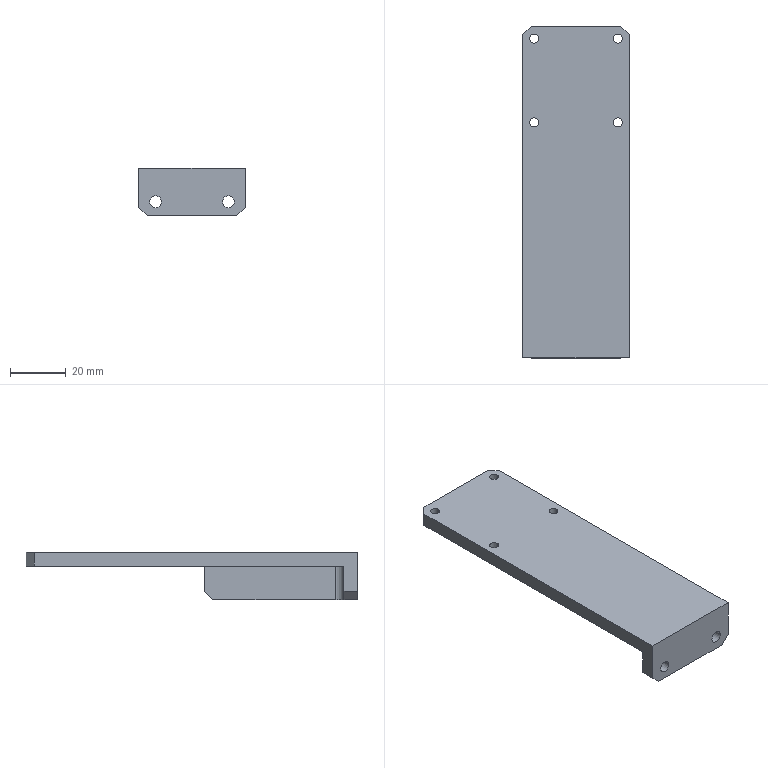NC program | NX | posted with a generic post | part box 38.1 x 118.8 x 17 mm
Lines 1974 to 2704 of 2704:
(ZLEVEL_PROFILE_1 , TOOL : D6R0.5)
N3916 T16 M6
N3918 G54
N3920 G17 G0 G90 X-2.413 Y7.413 S9500 M3
N3922 G43 Z30. H16
N3924 Z2.929
N3926 G94 G1 Z-0.071 F3500.
N3928 G3 X-4.625 Y4.472 R3.
N3930 G1 X-4.622 Y4.301
N3932 Y-4.301
N3934 X-4.625 Y-4.472
N3936 X-4.587 Y-4.473 Z-0.106
N3938 X-4.554 Z-0.141
N3940 X-4.551 Y-4.301
N3942 Y4.301
N3944 X-4.554 Y4.473
N3946 X-4.516 Z-0.177
N3948 X-4.483 Z-0.212
N3950 X-4.481 Y4.
N3952 Y-4.
N3954 X-4.483 Y-4.473
N3956 X-4.445 Z-0.247
N3958 X-4.413 Y-4.474 Z-0.283
N3960 X-4.41 Y-4.
N3962 Y4.
N3964 X-4.413 Y4.473
N3966 X-4.375 Y4.474 Z-0.318
N3968 X-4.342 Z-0.354
N3970 X-4.339 Y4.
N3972 Y-4.
N3974 X-4.342 Y-4.474
N3976 X-4.304 Z-0.389
N3978 X-4.271 Z-0.424
N3980 X-4.269 Y-4.
N3982 Y4.
N3984 X-4.271 Y4.474
N3986 X-4.233 Z-0.46
N3988 X-4.2 Y4.475 Z-0.495
N3990 X-4.198 Y4.
N3992 Y-4.
N3994 X-4.2 Y-4.475
N3996 X-4.163 Z-0.53
N3998 X-4.13 Z-0.566
N4000 X-4.127 Y-4.
N4002 Y4.
N4004 X-4.13 Y4.475
N4006 X-4.092 Z-0.601
N4008 X-4.059 Z-0.636
N4010 X-4.056 Y4.
N4012 Y-4.
N4014 X-4.059 Y-4.475
N4016 X-4.021 Y-4.476 Z-0.672
N4018 X-3.988 Z-0.707
N4020 X-3.986 Y-4.
N4022 Y4.
N4024 X-3.988 Y4.476
N4026 X-3.95 Z-0.742
N4028 X-3.918 Z-0.778
N4030 X-3.915 Y4.
N4032 Y-4.
N4034 X-3.918 Y-4.476
N4036 X-3.88 Z-0.813
N4038 X-3.847 Y-4.477 Z-0.849
N4040 X-3.844 Y-4.
N4042 Y4.
N4044 X-3.847 Y4.477
N4046 X-3.809 Z-0.884
N4048 X-3.776 Z-0.919
N4050 X-3.774 Y4.
N4052 Y-4.
N4054 X-3.776 Y-4.477
N4056 X-3.738 Z-0.955
N4058 X-3.705 Z-0.99
N4060 X-3.703 Y-4.
N4062 Y4.
N4064 X-3.705 Y4.477
N4066 X-3.668 Y4.478 Z-1.025
N4068 X-3.635 Z-1.061
N4070 X-3.632 Y4.
N4072 Y-4.
N4074 X-3.635 Y-4.478
N4076 X-3.597 Z-1.096
N4078 X-3.564 Z-1.131
N4080 X-3.562 Y-4.
N4082 Y4.
N4084 X-3.564 Y4.478
N4086 X-3.526 Z-1.167
N4088 X-3.493 Z-1.202
N4090 X-3.491 Y4.
N4092 Y-4.
N4094 X-3.493 Y-4.478
N4096 X-3.455 Z-1.237
N4098 X-3.423 Z-1.273
N4100 X-3.42 Y-4.
N4102 Y4.
N4104 X-3.423 Y4.478
N4106 X-3.385 Z-1.308
N4108 X-3.352 Z-1.344
N4110 X-3.349 Y4.
N4112 Y-4.
N4114 X-3.352 Y-4.478
N4116 X-3.314 Z-1.379
N4118 X-3.281 Z-1.414
N4120 X-3.279 Y-4.
N4122 Y4.
N4124 X-3.281 Y4.478
N4126 X-3.243 Z-1.45
N4128 X-3.21 Z-1.485
N4130 X-3.208 Y4.
N4132 Y-4.
N4134 X-3.21 Y-4.478
N4136 X-3.173 Z-1.52
N4138 X-3.14 Z-1.556
N4140 X-3.137 Y-4.
N4142 Y4.
N4144 X-3.14 Y4.478
N4146 X-3.102 Z-1.591
N4148 X-3.069 Z-1.626
N4150 X-3.067 Y4.
N4152 Y-4.
N4154 X-3.069 Y-4.478
N4156 X-3.031 Z-1.662
N4158 X-2.998 Z-1.697
N4160 X-2.996 Y-4.
N4162 Y4.
N4164 X-2.998 Y4.478
N4166 X-2.96 Z-1.732
N4168 X-2.928 Z-1.768
N4170 X-2.925 Y4.
N4172 Y-4.
N4174 X-2.928 Y-4.478
N4176 X-2.89 Z-1.803
N4178 X-2.857 Z-1.838
N4180 X-2.854 Y-4.
N4182 Y4.
N4184 X-2.857 Y4.478
N4186 X-2.819 Z-1.874
N4188 X-2.786 Z-1.909
N4190 X-2.784 Y4.
N4192 Y-4.
N4194 X-2.786 Y-4.478
N4196 X-2.748 Z-1.945
N4198 X-2.716 Z-1.98
N4200 X-2.713 Y-4.
N4202 Y4.
N4204 X-2.716 Y4.478
N4206 X-2.678 Z-2.015
N4208 X-2.645 Z-2.051
N4210 X-2.642 Y4.
N4212 Y-4.
N4214 X-2.645 Y-4.478
N4216 X-2.607 Z-2.086
N4218 X-2.574 Z-2.121
N4220 X-2.572 Y-4.
N4222 Y4.
N4224 X-2.574 Y4.478
N4226 X-2.536 Z-2.157
N4228 X-2.503 Z-2.192
N4230 X-2.501 Y4.
N4232 Y-4.
N4234 X-2.503 Y-4.478
N4236 X-2.466 Y-4.477 Z-2.227
N4238 X-2.433 Z-2.263
N4240 X-2.43 Y-4.
N4242 Y4.
N4244 X-2.433 Y4.477
N4246 X-2.395 Z-2.298
N4248 X-2.362 Z-2.333
N4250 X-2.359 Y4.
N4252 Y-4.
N4254 X-2.362 Y-4.477
N4256 X-2.324 Z-2.369
N4258 X-2.291 Z-2.404
N4260 X-2.289 Y-4.
N4262 Y4.
N4264 X-2.291 Y4.477
N4266 X-2.253 Z-2.44
N4268 X-2.221 Y4.476 Z-2.475
N4270 X-2.218 Y4.
N4272 Y-4.
N4274 X-2.221 Y-4.476
N4276 X-2.183 Z-2.51
N4278 X-2.15 Z-2.546
N4280 X-2.147 Y-4.
N4282 Y4.
N4284 X-2.15 Y4.476
N4286 X-2.112 Z-2.581
N4288 X-2.079 Z-2.616
N4290 X-2.077 Y4.
N4292 Y-4.
N4294 X-2.079 Y-4.476
N4296 X-2.041 Y-4.475 Z-2.652
N4298 X-2.008 Z-2.687
N4300 X-2.006 Y-4.
N4302 Y4.
N4304 X-2.008 Y4.475
N4306 X-1.971 Z-2.722
N4308 X-1.938 Z-2.758
N4310 X-1.935 Y4.
N4312 Y-4.
N4314 X-1.938 Y-4.475
N4316 X-1.9 Z-2.793
N4318 X-1.867 Y-4.474 Z-2.828
N4320 X-1.864 Y-4.
N4322 Y4.
N4324 X-1.867 Y4.474
N4326 X-1.829 Z-2.864
N4328 X-1.796 Z-2.899
N4330 X-1.794 Y4.
N4332 Y-4.
N4334 X-1.796 Y-4.474
N4336 X-1.758 Z-2.934
N4338 X-1.726 Z-2.97
N4340 X-1.723 Y-4.
N4342 Y4.
N4344 X-1.726 Y4.474
N4346 X-1.688 Y4.473 Z-3.005
N4348 X-1.655 Z-3.041
N4350 X-1.652 Y4.
N4352 Y-4.
N4354 X-1.655 Y-4.473
N4356 X-1.617 Z-3.076
N4358 X-1.584 Z-3.111
N4360 X-1.582 Y-4.
N4362 Y4.
N4364 X-1.584 Y4.473
N4366 X-1.546 Z-3.147
N4368 X-1.514 Y4.472 Z-3.182
N4370 X-1.511 Y4.301
N4372 Y-4.301
N4374 X-1.514 Y-4.472
N4376 X-1.476 Z-3.217
N4378 X-1.443 Z-3.253
N4380 X-1.44 Y-4.301
N4382 Y4.301
N4384 X-1.443 Y4.472
N4386 X-1.409 Z-3.284
N4388 X-1.381 Z-3.315
N4390 X-1.378 Y4.301
N4392 Y-4.301
N4394 X-1.381 Y-4.472
N4396 X-1.347 Y-4.471 Z-3.345
N4398 X-1.319 Z-3.376
N4400 X-1.317 Y-4.301
N4402 Y4.301
N4404 X-1.319 Y4.471
N4406 X-1.256 Y4.391 Z-3.438
N4408 X-1.255 Y4.301
N4410 Y-4.301
N4412 X-1.256 Y-4.391
N4414 G3 X0.989 Y-7.351 R3.
N4416 G1 Z-0.438
N4418 G0 Z30.
N4420 X-51.024 Y-21.059
N4422 Z2.929
N4424 G1 Z-0.071
N4426 G3 X-53.968 Y-18.826 R3.
N4428 G1 X-54.106 Y-18.828
N4430 X-59.815 Y-18.827
N4432 X-59.869 Y-18.898 Z-0.141
N4434 X-54.106 Y-18.899
N4436 X-53.93 Y-18.896
N4438 X-53.928 Y-18.934 Z-0.177
N4440 X-53.927 Y-18.967 Z-0.212
N4442 X-54.4 Y-18.969
N4444 X-59.4
N4446 X-59.873 Y-18.968
N4448 Y-19.005 Z-0.247
N4450 X-59.874 Y-19.039 Z-0.283
N4452 X-59.4 Y-19.04
N4454 X-54.4
N4456 X-53.927 Y-19.037
N4458 X-53.926 Y-19.075 Z-0.318
N4460 Y-19.108 Z-0.354
N4462 X-54.4 Y-19.111
N4464 X-59.4
N4466 X-59.874 Y-19.11
N4468 Y-19.146 Z-0.389
N4470 Y-19.18 Z-0.424
N4472 X-59.4 Y-19.181
N4474 X-54.4
N4476 X-53.926 Y-19.179
N4478 Y-19.217 Z-0.46
N4480 X-53.925 Y-19.25 Z-0.495
N4482 X-54.4 Y-19.252
N4484 X-59.4
N4486 X-59.875 Y-19.251
N4488 Y-19.287 Z-0.53
N4490 Y-19.322 Z-0.566
N4492 X-59.4 Y-19.323
N4494 X-54.4
N4496 X-53.925 Y-19.32
N4498 Y-19.358 Z-0.601
N4500 Y-19.391 Z-0.636
N4502 X-54.4 Y-19.394
N4504 X-59.4
N4506 X-59.875 Y-19.393
N4508 X-59.876 Y-19.429 Z-0.672
N4510 Y-19.463 Z-0.707
N4512 X-59.4 Y-19.464
N4514 X-54.4
N4516 X-53.924 Y-19.462
N4518 Y-19.5 Z-0.742
N4520 Y-19.532 Z-0.778
N4522 X-54.4 Y-19.535
N4524 X-59.4
N4526 X-59.876 Y-19.534
N4528 Y-19.57 Z-0.813
N4530 X-59.877 Y-19.605 Z-0.849
N4532 X-59.4 Y-19.606
N4534 X-54.4
N4536 X-53.923 Y-19.603
N4538 Y-19.641 Z-0.884
N4540 Y-19.674 Z-0.919
N4542 X-54.4 Y-19.676
N4544 X-59.4
N4546 X-59.877 Y-19.675
N4548 Y-19.712 Z-0.955
N4550 Y-19.746 Z-0.99
N4552 X-59.4 Y-19.747
N4554 X-54.4
N4556 X-53.923 Y-19.745
N4558 X-53.922 Y-19.782 Z-1.025
N4560 Y-19.815 Z-1.061
N4562 X-54.4 Y-19.818
N4564 X-59.4
N4566 X-59.878 Y-19.817
N4568 Y-19.853 Z-1.096
N4570 Y-19.888 Z-1.131
N4572 X-59.4
N4574 X-54.4
N4576 X-53.922 Y-19.886
N4578 Y-19.924 Z-1.167
N4580 Y-19.957 Z-1.202
N4582 X-54.4 Y-19.959
N4584 X-59.4
N4586 X-59.878 Y-19.958
N4588 Y-19.995 Z-1.237
N4590 Y-20.029 Z-1.273
N4592 X-59.4 Y-20.03
N4594 X-54.4
N4596 X-53.922 Y-20.027
N4598 Y-20.065 Z-1.308
N4600 Y-20.098 Z-1.344
N4602 X-54.4 Y-20.101
N4604 X-59.4
N4606 X-59.878 Y-20.1
N4608 Y-20.136 Z-1.379
N4610 Y-20.17 Z-1.414
N4612 X-59.4 Y-20.171
N4614 X-54.4
N4616 X-53.922 Y-20.169
N4618 Y-20.207 Z-1.45
N4620 Y-20.24 Z-1.485
N4622 X-54.4 Y-20.242
N4624 X-59.4
N4626 X-59.878 Y-20.241
N4628 Y-20.277 Z-1.52
N4630 Y-20.312 Z-1.556
N4632 X-59.4 Y-20.313
N4634 X-54.4
N4636 X-53.922 Y-20.31
N4638 Y-20.348 Z-1.591
N4640 Y-20.381 Z-1.626
N4642 X-54.4 Y-20.383
N4644 X-59.4
N4646 X-59.878
N4648 Y-20.419 Z-1.662
N4650 Y-20.453 Z-1.697
N4652 X-59.4 Y-20.454
N4654 X-54.4
N4656 X-53.922 Y-20.452
N4658 Y-20.49 Z-1.732
N4660 Y-20.522 Z-1.768
N4662 X-54.4 Y-20.525
N4664 X-59.4
N4666 X-59.878 Y-20.524
N4668 Y-20.56 Z-1.803
N4670 Y-20.595 Z-1.838
N4672 X-59.4 Y-20.596
N4674 X-54.4
N4676 X-53.922 Y-20.593
N4678 Y-20.631 Z-1.874
N4680 Y-20.664 Z-1.909
N4682 X-54.4 Y-20.666
N4684 X-59.4
N4686 X-59.878 Y-20.665
N4688 Y-20.702 Z-1.945
N4690 Y-20.736 Z-1.98
N4692 X-59.4 Y-20.737
N4694 X-54.4
N4696 X-53.922 Y-20.735
N4698 Y-20.772 Z-2.015
N4700 Y-20.805 Z-2.051
N4702 X-54.4 Y-20.808
N4704 X-59.4
N4706 X-59.878 Y-20.807
N4708 Y-20.843 Z-2.086
N4710 Y-20.878 Z-2.121
N4712 X-59.4
N4714 X-54.4
N4716 X-53.922 Y-20.876
N4718 Y-20.914 Z-2.157
N4720 Y-20.947 Z-2.192
N4722 X-54.4 Y-20.949
N4724 X-59.4
N4726 X-59.878 Y-20.948
N4728 Y-20.984 Z-2.227
N4730 Y-21.019 Z-2.263
N4732 X-59.4 Y-21.02
N4734 X-54.4
N4736 X-53.922 Y-21.017
N4738 X-53.923 Y-21.055 Z-2.298
N4740 Y-21.088 Z-2.333
N4742 X-54.4 Y-21.091
N4744 X-59.4
N4746 X-59.877 Y-21.09
N4748 Y-21.126 Z-2.369
N4750 Y-21.16 Z-2.404
N4752 X-59.4 Y-21.161
N4754 X-54.4
N4756 X-53.923 Y-21.159
N4758 Y-21.197 Z-2.44
N4760 X-53.924 Y-21.23 Z-2.475
N4762 X-54.4 Y-21.232
N4764 X-59.4
N4766 X-59.876 Y-21.231
N4768 Y-21.267 Z-2.51
N4770 Y-21.302 Z-2.546
N4772 X-59.4 Y-21.303
N4774 X-54.4
N4776 X-53.924 Y-21.3
N4778 Y-21.338 Z-2.581
N4780 Y-21.371 Z-2.616
N4782 X-54.4 Y-21.373
N4784 X-59.4
N4786 X-59.876 Y-21.372
N4788 X-59.875 Y-21.409 Z-2.652
N4790 Y-21.443 Z-2.687
N4792 X-59.4 Y-21.444
N4794 X-54.4
N4796 X-53.925 Y-21.442
N4798 Y-21.479 Z-2.722
N4800 Y-21.512 Z-2.758
N4802 X-54.4 Y-21.515
N4804 X-59.4
N4806 X-59.875 Y-21.514
N4808 Y-21.55 Z-2.793
N4810 Y-21.585 Z-2.828
N4812 X-59.4 Y-21.586
N4814 X-54.4
N4816 X-53.926 Y-21.583
N4818 Y-21.621 Z-2.864
N4820 Y-21.654 Z-2.899
N4822 X-54.4 Y-21.656
N4824 X-59.4
N4826 X-59.874 Y-21.655
N4828 Y-21.692 Z-2.934
N4830 Y-21.726 Z-2.97
N4832 X-59.4 Y-21.727
N4834 X-54.4
N4836 X-53.926 Y-21.724
N4838 X-53.927 Y-21.762 Z-3.005
N4840 Y-21.795 Z-3.041
N4842 X-54.4 Y-21.798
N4844 X-59.4
N4846 X-59.873 Y-21.797
N4848 Y-21.833 Z-3.076
N4850 Y-21.867 Z-3.111
N4852 X-59.4 Y-21.868
N4854 X-54.4
N4856 X-53.927 Y-21.866
N4858 Y-21.904 Z-3.147
N4860 X-53.928 Y-21.937 Z-3.182
N4862 X-54.106 Y-21.939
N4864 X-59.873 Y-21.938
N4866 X-59.872 Y-21.974 Z-3.217
N4868 Y-22.009 Z-3.253
N4870 X-54.106 Y-22.01
N4872 X-53.928 Y-22.007
N4874 X-53.974 Y-22.07 Z-3.315
N4876 X-54.106 Y-22.072
N4878 X-59.806 Y-22.071
N4880 X-59.735 Y-22.133 Z-3.376
N4882 X-54.023 Y-22.132
N4884 X-54.072 Y-22.195 Z-3.438
N4886 X-59.664
N4888 G3 X-62.588 Y-24.526 R3.
N4890 G1 Z-0.438
N4892 G0 Z30.
N4894 X-62.722 Y21.085
N4896 Z2.929
N4898 G1 Z-0.071
N4900 G3 X-59.815 Y18.827 R3.
N4902 G1 X-54.106 Y18.828
N4904 X-53.968 Y18.826
N4906 X-53.93 Y18.896 Z-0.141
N4908 X-54.106 Y18.899
N4910 X-59.869 Y18.898
N4912 X-59.871 Y18.934 Z-0.177
N4914 X-59.873 Y18.968 Z-0.212
N4916 X-59.4 Y18.969
N4918 X-54.4
N4920 X-53.927 Y18.967
N4922 Y19.005 Z-0.247
N4924 Y19.037 Z-0.283
N4926 X-54.4 Y19.04
N4928 X-59.4
N4930 X-59.874 Y19.039
N4932 Y19.075 Z-0.318
N4934 Y19.11 Z-0.354
N4936 X-59.4 Y19.111
N4938 X-54.4
N4940 X-53.926 Y19.108
N4942 Y19.146 Z-0.389
N4944 Y19.179 Z-0.424
N4946 X-54.4 Y19.181
N4948 X-59.4
N4950 X-59.874 Y19.18
N4952 X-59.875 Y19.217 Z-0.46
N4954 Y19.251 Z-0.495
N4956 X-59.4 Y19.252
N4958 X-54.4
N4960 X-53.925 Y19.25
N4962 Y19.287 Z-0.53
N4964 Y19.32 Z-0.566
N4966 X-54.4 Y19.323
N4968 X-59.4
N4970 X-59.875 Y19.322
N4972 Y19.358 Z-0.601
N4974 Y19.393 Z-0.636
N4976 X-59.4 Y19.394
N4978 X-54.4
N4980 X-53.925 Y19.391
N4982 X-53.924 Y19.429 Z-0.672
N4984 Y19.462 Z-0.707
N4986 X-54.4 Y19.464
N4988 X-59.4
N4990 X-59.876 Y19.463
N4992 Y19.5 Z-0.742
N4994 Y19.534 Z-0.778
N4996 X-59.4 Y19.535
N4998 X-54.4
N5000 X-53.924 Y19.532
N5002 Y19.57 Z-0.813
N5004 X-53.923 Y19.603 Z-0.849
N5006 X-54.4 Y19.606
N5008 X-59.4
N5010 X-59.877 Y19.605
N5012 Y19.641 Z-0.884
N5014 Y19.675 Z-0.919
N5016 X-59.4 Y19.676
N5018 X-54.4
N5020 X-53.923 Y19.674
N5022 Y19.712 Z-0.955
N5024 Y19.745 Z-0.99
N5026 X-54.4 Y19.747
N5028 X-59.4
N5030 X-59.877 Y19.746
N5032 Y19.782 Z-1.025
N5034 X-59.878 Y19.817 Z-1.061
N5036 X-59.4 Y19.818
N5038 X-54.4
N5040 X-53.922 Y19.815
N5042 Y19.853 Z-1.096
N5044 Y19.886 Z-1.131
N5046 X-54.4 Y19.888
N5048 X-59.4
N5050 X-59.878
N5052 Y19.924 Z-1.167
N5054 Y19.958 Z-1.202
N5056 X-59.4 Y19.959
N5058 X-54.4
N5060 X-53.922 Y19.957
N5062 Y19.995 Z-1.237
N5064 Y20.027 Z-1.273
N5066 X-54.4 Y20.03
N5068 X-59.4
N5070 X-59.878 Y20.029
N5072 Y20.065 Z-1.308
N5074 Y20.1 Z-1.344
N5076 X-59.4 Y20.101
N5078 X-54.4
N5080 X-53.922 Y20.098
N5082 Y20.136 Z-1.379
N5084 Y20.169 Z-1.414
N5086 X-54.4 Y20.171
N5088 X-59.4
N5090 X-59.878 Y20.17
N5092 Y20.207 Z-1.45
N5094 Y20.241 Z-1.485
N5096 X-59.4 Y20.242
N5098 X-54.4
N5100 X-53.922 Y20.24
N5102 Y20.277 Z-1.52
N5104 Y20.31 Z-1.556
N5106 X-54.4 Y20.313
N5108 X-59.4
N5110 X-59.878 Y20.312
N5112 Y20.348 Z-1.591
N5114 Y20.383 Z-1.626
N5116 X-59.4
N5118 X-54.4
N5120 X-53.922 Y20.381
N5122 Y20.419 Z-1.662
N5124 Y20.452 Z-1.697
N5126 X-54.4 Y20.454
N5128 X-59.4
N5130 X-59.878 Y20.453
N5132 Y20.49 Z-1.732
N5134 Y20.524 Z-1.768
N5136 X-59.4 Y20.525
N5138 X-54.4
N5140 X-53.922 Y20.522
N5142 Y20.56 Z-1.803
N5144 Y20.593 Z-1.838
N5146 X-54.4 Y20.596
N5148 X-59.4
N5150 X-59.878 Y20.595
N5152 Y20.631 Z-1.874
N5154 Y20.665 Z-1.909
N5156 X-59.4 Y20.666
N5158 X-54.4
N5160 X-53.922 Y20.664
N5162 Y20.702 Z-1.945
N5164 Y20.735 Z-1.98
N5166 X-54.4 Y20.737
N5168 X-59.4
N5170 X-59.878 Y20.736
N5172 Y20.772 Z-2.015
N5174 Y20.807 Z-2.051
N5176 X-59.4 Y20.808
N5178 X-54.4
N5180 X-53.922 Y20.805
N5182 Y20.843 Z-2.086
N5184 Y20.876 Z-2.121
N5186 X-54.4 Y20.878
N5188 X-59.4
N5190 X-59.878
N5192 Y20.914 Z-2.157
N5194 Y20.948 Z-2.192
N5196 X-59.4 Y20.949
N5198 X-54.4
N5200 X-53.922 Y20.947
N5202 Y20.984 Z-2.227
N5204 Y21.017 Z-2.263
N5206 X-54.4 Y21.02
N5208 X-59.4
N5210 X-59.878 Y21.019
N5212 X-59.877 Y21.055 Z-2.298
N5214 Y21.09 Z-2.333
N5216 X-59.4 Y21.091
N5218 X-54.4
N5220 X-53.923 Y21.088
N5222 Y21.126 Z-2.369
N5224 Y21.159 Z-2.404
N5226 X-54.4 Y21.161
N5228 X-59.4
N5230 X-59.877 Y21.16
N5232 Y21.197 Z-2.44
N5234 X-59.876 Y21.231 Z-2.475
N5236 X-59.4 Y21.232
N5238 X-54.4
N5240 X-53.924 Y21.23
N5242 Y21.267 Z-2.51
N5244 Y21.3 Z-2.546
N5246 X-54.4 Y21.303
N5248 X-59.4
N5250 X-59.876 Y21.302
N5252 Y21.338 Z-2.581
N5254 Y21.372 Z-2.616
N5256 X-59.4 Y21.373
N5258 X-54.4
N5260 X-53.924 Y21.371
N5262 X-53.925 Y21.409 Z-2.652
N5264 Y21.442 Z-2.687
N5266 X-54.4 Y21.444
N5268 X-59.4
N5270 X-59.875 Y21.443
N5272 Y21.479 Z-2.722
N5274 Y21.514 Z-2.758
N5276 X-59.4 Y21.515
N5278 X-54.4
N5280 X-53.925 Y21.512
N5282 Y21.55 Z-2.793
N5284 X-53.926 Y21.583 Z-2.828
N5286 X-54.4 Y21.586
N5288 X-59.4
N5290 X-59.875 Y21.585
N5292 X-59.874 Y21.621 Z-2.864
N5294 Y21.655 Z-2.899
N5296 X-59.4 Y21.656
N5298 X-54.4
N5300 X-53.926 Y21.654
N5302 Y21.692 Z-2.934
N5304 Y21.724 Z-2.97
N5306 X-54.4 Y21.727
N5308 X-59.4
N5310 X-59.874 Y21.726
N5312 Y21.762 Z-3.005
N5314 X-59.873 Y21.797 Z-3.041
N5316 X-59.4 Y21.798
N5318 X-54.4
N5320 X-53.927 Y21.795
N5322 Y21.833 Z-3.076
N5324 Y21.866 Z-3.111
N5326 X-54.4 Y21.868
N5328 X-59.4
N5330 X-59.873 Y21.867
N5332 Y21.904 Z-3.147
N5334 Y21.938 Z-3.182
N5336 X-54.106 Y21.939
N5338 X-53.928 Y21.937
N5340 Y21.974 Z-3.217
N5342 Y22.007 Z-3.253
N5344 X-54.106 Y22.01
N5346 X-59.872 Y22.009
N5348 X-59.806 Y22.071 Z-3.315
N5350 X-54.106 Y22.072
N5352 X-53.974 Y22.07
N5354 X-54.023 Y22.132 Z-3.376
N5356 X-59.735 Y22.133
N5358 X-59.664 Y22.195 Z-3.438
N5360 X-54.072
N5362 G3 X-51.155 Y24.497 R3.
N5364 G1 Z-0.438
N5366 G0 Z30.
N5368 M5
N5370 M2